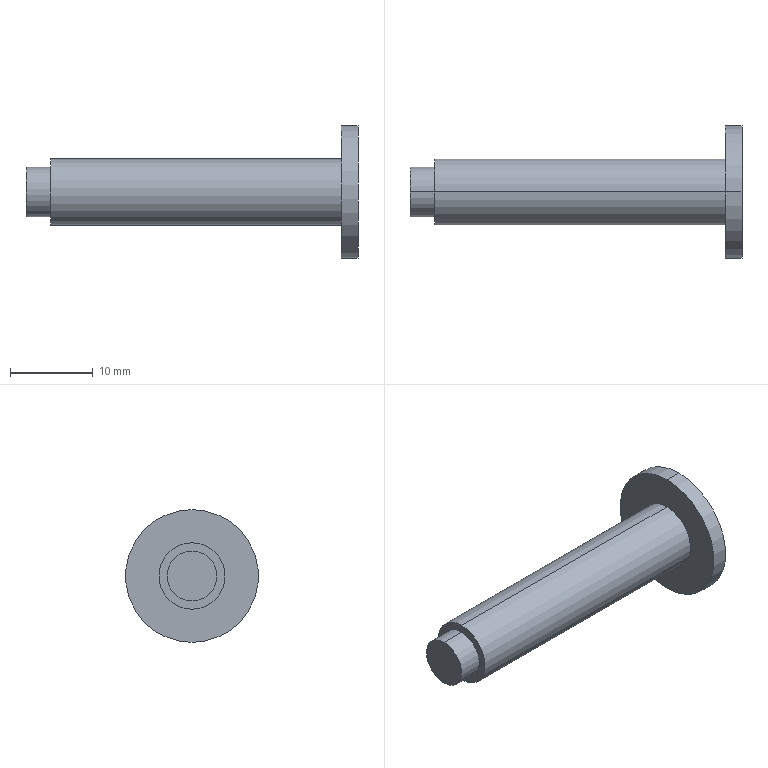Part | SolidWorks | features Revolution 1 | 1 solid | 10 faces | box 40 x 16 x 16 mm | volume 2246 mm3 | cylinder 6 | plane 4 | commonest cylinder face diameters 6 x2 8 x2 16 x2
STEP:
#1=CARTESIAN_POINT('',(3.,0.,-4.));
#2=VERTEX_POINT('',#1);
#3=CARTESIAN_POINT('',(3.,0.,4.));
#4=VERTEX_POINT('',#3);
#5=CARTESIAN_POINT('',(3.,0.,0.));
#6=DIRECTION('',(1.,0.,0.));
#7=DIRECTION('',(0.,0.,-1.));
#8=AXIS2_PLACEMENT_3D('',#5,#6,#7);
#9=CIRCLE('',#8,4.);
#10=EDGE_CURVE('',#2,#4,#9,.T.);
#11=ORIENTED_EDGE('',*,*,#10,.T.);
#12=CARTESIAN_POINT('',(38.,0.,4.));
#13=VERTEX_POINT('',#12);
#14=CARTESIAN_POINT('',(40.,0.,4.));
#15=DIRECTION('',(1.,0.,0.));
#16=VECTOR('',#15,1000.);
#17=LINE('',#14,#16);
#18=EDGE_CURVE('',#4,#13,#17,.T.);
#19=ORIENTED_EDGE('',*,*,#18,.T.);
#20=CARTESIAN_POINT('',(38.,0.,-4.));
#21=VERTEX_POINT('',#20);
#22=CARTESIAN_POINT('',(38.,0.,0.));
#23=DIRECTION('',(1.,0.,0.));
#24=DIRECTION('',(0.,0.,-1.));
#25=AXIS2_PLACEMENT_3D('',#22,#23,#24);
#26=CIRCLE('',#25,4.);
#27=EDGE_CURVE('',#21,#13,#26,.T.);
#28=ORIENTED_EDGE('',*,*,#27,.F.);
#29=CARTESIAN_POINT('',(40.,0.,-4.));
#30=DIRECTION('',(1.,0.,0.));
#31=VECTOR('',#30,1000.);
#32=LINE('',#29,#31);
#33=EDGE_CURVE('',#2,#21,#32,.T.);
#34=ORIENTED_EDGE('',*,*,#33,.F.);
#35=EDGE_LOOP('',(#11,#19,#28,#34));
#36=FACE_OUTER_BOUND('',#35,.T.);
#37=CARTESIAN_POINT('',(40.,0.,0.));
#38=DIRECTION('',(1.,0.,0.));
#39=DIRECTION('',(0.,0.,-1.));
#40=AXIS2_PLACEMENT_3D('',#37,#38,#39);
#41=CYLINDRICAL_SURFACE('',#40,4.);
#42=ADVANCED_FACE('',(#36),#41,.T.);
#43=CARTESIAN_POINT('',(38.,0.,-8.));
#44=VERTEX_POINT('',#43);
#45=CARTESIAN_POINT('',(38.,0.,8.));
#46=VERTEX_POINT('',#45);
#47=CARTESIAN_POINT('',(38.,0.,0.));
#48=DIRECTION('',(1.,0.,0.));
#49=DIRECTION('',(0.,0.,-1.));
#50=AXIS2_PLACEMENT_3D('',#47,#48,#49);
#51=CIRCLE('',#50,8.);
#52=EDGE_CURVE('',#44,#46,#51,.T.);
#53=ORIENTED_EDGE('',*,*,#52,.T.);
#54=CARTESIAN_POINT('',(40.,0.,8.));
#55=VERTEX_POINT('',#54);
#56=CARTESIAN_POINT('',(40.,0.,8.));
#57=DIRECTION('',(1.,0.,0.));
#58=VECTOR('',#57,1000.);
#59=LINE('',#56,#58);
#60=EDGE_CURVE('',#46,#55,#59,.T.);
#61=ORIENTED_EDGE('',*,*,#60,.T.);
#62=CARTESIAN_POINT('',(40.,0.,-8.));
#63=VERTEX_POINT('',#62);
#64=CARTESIAN_POINT('',(40.,0.,0.));
#65=DIRECTION('',(1.,0.,0.));
#66=DIRECTION('',(0.,0.,-1.));
#67=AXIS2_PLACEMENT_3D('',#64,#65,#66);
#68=CIRCLE('',#67,8.);
#69=EDGE_CURVE('',#63,#55,#68,.T.);
#70=ORIENTED_EDGE('',*,*,#69,.F.);
#71=CARTESIAN_POINT('',(40.,0.,-8.));
#72=DIRECTION('',(1.,0.,0.));
#73=VECTOR('',#72,1000.);
#74=LINE('',#71,#73);
#75=EDGE_CURVE('',#44,#63,#74,.T.);
#76=ORIENTED_EDGE('',*,*,#75,.F.);
#77=EDGE_LOOP('',(#53,#61,#70,#76));
#78=FACE_OUTER_BOUND('',#77,.T.);
#79=CARTESIAN_POINT('',(40.,0.,0.));
#80=DIRECTION('',(1.,0.,0.));
#81=DIRECTION('',(0.,0.,-1.));
#82=AXIS2_PLACEMENT_3D('',#79,#80,#81);
#83=CYLINDRICAL_SURFACE('',#82,8.);
#84=ADVANCED_FACE('',(#78),#83,.T.);
#85=CARTESIAN_POINT('',(0.,0.,-3.));
#86=VERTEX_POINT('',#85);
#87=CARTESIAN_POINT('',(0.,0.,3.));
#88=VERTEX_POINT('',#87);
#89=CARTESIAN_POINT('',(0.,0.,0.));
#90=DIRECTION('',(1.,0.,0.));
#91=DIRECTION('',(0.,0.,-1.));
#92=AXIS2_PLACEMENT_3D('',#89,#90,#91);
#93=CIRCLE('',#92,3.);
#94=EDGE_CURVE('',#86,#88,#93,.T.);
#95=ORIENTED_EDGE('',*,*,#94,.T.);
#96=CARTESIAN_POINT('',(3.,0.,3.));
#97=VERTEX_POINT('',#96);
#98=CARTESIAN_POINT('',(40.,0.,3.));
#99=DIRECTION('',(1.,0.,0.));
#100=VECTOR('',#99,1000.);
#101=LINE('',#98,#100);
#102=EDGE_CURVE('',#88,#97,#101,.T.);
#103=ORIENTED_EDGE('',*,*,#102,.T.);
#104=CARTESIAN_POINT('',(3.,0.,-3.));
#105=VERTEX_POINT('',#104);
#106=CARTESIAN_POINT('',(3.,0.,0.));
#107=DIRECTION('',(1.,0.,0.));
#108=DIRECTION('',(0.,0.,-1.));
#109=AXIS2_PLACEMENT_3D('',#106,#107,#108);
#110=CIRCLE('',#109,3.);
#111=EDGE_CURVE('',#105,#97,#110,.T.);
#112=ORIENTED_EDGE('',*,*,#111,.F.);
#113=CARTESIAN_POINT('',(40.,0.,-3.));
#114=DIRECTION('',(1.,0.,0.));
#115=VECTOR('',#114,1000.);
#116=LINE('',#113,#115);
#117=EDGE_CURVE('',#86,#105,#116,.T.);
#118=ORIENTED_EDGE('',*,*,#117,.F.);
#119=EDGE_LOOP('',(#95,#103,#112,#118));
#120=FACE_OUTER_BOUND('',#119,.T.);
#121=CARTESIAN_POINT('',(40.,0.,0.));
#122=DIRECTION('',(1.,0.,0.));
#123=DIRECTION('',(0.,0.,-1.));
#124=AXIS2_PLACEMENT_3D('',#121,#122,#123);
#125=CYLINDRICAL_SURFACE('',#124,3.);
#126=ADVANCED_FACE('',(#120),#125,.T.);
#127=ORIENTED_EDGE('',*,*,#102,.F.);
#128=CARTESIAN_POINT('',(0.,0.,0.));
#129=DIRECTION('',(1.,0.,0.));
#130=DIRECTION('',(0.,0.,-1.));
#131=AXIS2_PLACEMENT_3D('',#128,#129,#130);
#132=CIRCLE('',#131,3.);
#133=EDGE_CURVE('',#88,#86,#132,.T.);
#134=ORIENTED_EDGE('',*,*,#133,.T.);
#135=ORIENTED_EDGE('',*,*,#117,.T.);
#136=CARTESIAN_POINT('',(3.,0.,0.));
#137=DIRECTION('',(1.,0.,0.));
#138=DIRECTION('',(0.,0.,-1.));
#139=AXIS2_PLACEMENT_3D('',#136,#137,#138);
#140=CIRCLE('',#139,3.);
#141=EDGE_CURVE('',#97,#105,#140,.T.);
#142=ORIENTED_EDGE('',*,*,#141,.F.);
#143=EDGE_LOOP('',(#127,#134,#135,#142));
#144=FACE_OUTER_BOUND('',#143,.T.);
#145=CARTESIAN_POINT('',(40.,0.,0.));
#146=DIRECTION('',(1.,0.,0.));
#147=DIRECTION('',(0.,0.,-1.));
#148=AXIS2_PLACEMENT_3D('',#145,#146,#147);
#149=CYLINDRICAL_SURFACE('',#148,3.);
#150=ADVANCED_FACE('',(#144),#149,.T.);
#151=ORIENTED_EDGE('',*,*,#94,.F.);
#152=ORIENTED_EDGE('',*,*,#133,.F.);
#153=EDGE_LOOP('',(#151,#152));
#154=FACE_OUTER_BOUND('',#153,.T.);
#155=CARTESIAN_POINT('',(0.,0.,0.));
#156=DIRECTION('',(-1.,0.,0.));
#157=DIRECTION('',(0.,0.,1.));
#158=AXIS2_PLACEMENT_3D('',#155,#156,#157);
#159=PLANE('',#158);
#160=ADVANCED_FACE('',(#154),#159,.T.);
#161=ORIENTED_EDGE('',*,*,#69,.T.);
#162=CARTESIAN_POINT('',(40.,0.,0.));
#163=DIRECTION('',(1.,0.,0.));
#164=DIRECTION('',(0.,0.,-1.));
#165=AXIS2_PLACEMENT_3D('',#162,#163,#164);
#166=CIRCLE('',#165,8.);
#167=EDGE_CURVE('',#55,#63,#166,.T.);
#168=ORIENTED_EDGE('',*,*,#167,.T.);
#169=EDGE_LOOP('',(#161,#168));
#170=FACE_OUTER_BOUND('',#169,.T.);
#171=CARTESIAN_POINT('',(40.,8.,0.));
#172=DIRECTION('',(1.,0.,0.));
#173=DIRECTION('',(0.,0.,-1.));
#174=AXIS2_PLACEMENT_3D('',#171,#172,#173);
#175=PLANE('',#174);
#176=ADVANCED_FACE('',(#170),#175,.T.);
#177=ORIENTED_EDGE('',*,*,#60,.F.);
#178=CARTESIAN_POINT('',(38.,0.,0.));
#179=DIRECTION('',(1.,0.,0.));
#180=DIRECTION('',(0.,0.,-1.));
#181=AXIS2_PLACEMENT_3D('',#178,#179,#180);
#182=CIRCLE('',#181,8.);
#183=EDGE_CURVE('',#46,#44,#182,.T.);
#184=ORIENTED_EDGE('',*,*,#183,.T.);
#185=ORIENTED_EDGE('',*,*,#75,.T.);
#186=ORIENTED_EDGE('',*,*,#167,.F.);
#187=EDGE_LOOP('',(#177,#184,#185,#186));
#188=FACE_OUTER_BOUND('',#187,.T.);
#189=CARTESIAN_POINT('',(40.,0.,0.));
#190=DIRECTION('',(1.,0.,0.));
#191=DIRECTION('',(0.,0.,-1.));
#192=AXIS2_PLACEMENT_3D('',#189,#190,#191);
#193=CYLINDRICAL_SURFACE('',#192,8.);
#194=ADVANCED_FACE('',(#188),#193,.T.);
#195=ORIENTED_EDGE('',*,*,#27,.T.);
#196=CARTESIAN_POINT('',(38.,0.,0.));
#197=DIRECTION('',(1.,0.,0.));
#198=DIRECTION('',(0.,0.,-1.));
#199=AXIS2_PLACEMENT_3D('',#196,#197,#198);
#200=CIRCLE('',#199,4.);
#201=EDGE_CURVE('',#13,#21,#200,.T.);
#202=ORIENTED_EDGE('',*,*,#201,.T.);
#203=EDGE_LOOP('',(#195,#202));
#204=FACE_BOUND('',#203,.T.);
#205=ORIENTED_EDGE('',*,*,#52,.F.);
#206=ORIENTED_EDGE('',*,*,#183,.F.);
#207=EDGE_LOOP('',(#205,#206));
#208=FACE_OUTER_BOUND('',#207,.T.);
#209=CARTESIAN_POINT('',(38.,4.,0.));
#210=DIRECTION('',(-1.,0.,0.));
#211=DIRECTION('',(0.,0.,1.));
#212=AXIS2_PLACEMENT_3D('',#209,#210,#211);
#213=PLANE('',#212);
#214=ADVANCED_FACE('',(#204,#208),#213,.T.);
#215=ORIENTED_EDGE('',*,*,#18,.F.);
#216=CARTESIAN_POINT('',(3.,0.,0.));
#217=DIRECTION('',(1.,0.,0.));
#218=DIRECTION('',(0.,0.,-1.));
#219=AXIS2_PLACEMENT_3D('',#216,#217,#218);
#220=CIRCLE('',#219,4.);
#221=EDGE_CURVE('',#4,#2,#220,.T.);
#222=ORIENTED_EDGE('',*,*,#221,.T.);
#223=ORIENTED_EDGE('',*,*,#33,.T.);
#224=ORIENTED_EDGE('',*,*,#201,.F.);
#225=EDGE_LOOP('',(#215,#222,#223,#224));
#226=FACE_OUTER_BOUND('',#225,.T.);
#227=CARTESIAN_POINT('',(40.,0.,0.));
#228=DIRECTION('',(1.,0.,0.));
#229=DIRECTION('',(0.,0.,-1.));
#230=AXIS2_PLACEMENT_3D('',#227,#228,#229);
#231=CYLINDRICAL_SURFACE('',#230,4.);
#232=ADVANCED_FACE('',(#226),#231,.T.);
#233=ORIENTED_EDGE('',*,*,#111,.T.);
#234=ORIENTED_EDGE('',*,*,#141,.T.);
#235=EDGE_LOOP('',(#233,#234));
#236=FACE_BOUND('',#235,.T.);
#237=ORIENTED_EDGE('',*,*,#10,.F.);
#238=ORIENTED_EDGE('',*,*,#221,.F.);
#239=EDGE_LOOP('',(#237,#238));
#240=FACE_OUTER_BOUND('',#239,.T.);
#241=CARTESIAN_POINT('',(3.,3.,0.));
#242=DIRECTION('',(-1.,0.,0.));
#243=DIRECTION('',(0.,0.,1.));
#244=AXIS2_PLACEMENT_3D('',#241,#242,#243);
#245=PLANE('',#244);
#246=ADVANCED_FACE('',(#236,#240),#245,.T.);
#247=CLOSED_SHELL('',(#42,#84,#126,#150,#160,#176,#194,#214,#232,#246));
#248=MANIFOLD_SOLID_BREP('',#247);
#249=CARTESIAN_POINT('',(0.,0.,0.));
#250=DIRECTION('',(0.,0.,1.));
#251=DIRECTION('',(1.,0.,0.));
#252=AXIS2_PLACEMENT_3D('',#249,#250,#251);
#253=(LENGTH_UNIT()NAMED_UNIT(*)SI_UNIT(.MILLI.,.METRE.));
#254=UNCERTAINTY_MEASURE_WITH_UNIT(LENGTH_MEASURE(0.00001),#253,'','');
#255=(NAMED_UNIT(*)PLANE_ANGLE_UNIT()SI_UNIT($,.RADIAN.));
#256=(NAMED_UNIT(*)SI_UNIT($,.STERADIAN.)SOLID_ANGLE_UNIT());
#257=(GEOMETRIC_REPRESENTATION_CONTEXT(3)GLOBAL_UNCERTAINTY_ASSIGNED_CONTEXT((#254))GLOBAL_UNIT_ASSIGNED_CONTEXT((#253,#255,#256))REPRESENTATION_CONTEXT('',''));
#258=ADVANCED_BREP_SHAPE_REPRESENTATION('',(#248,#252),#257);